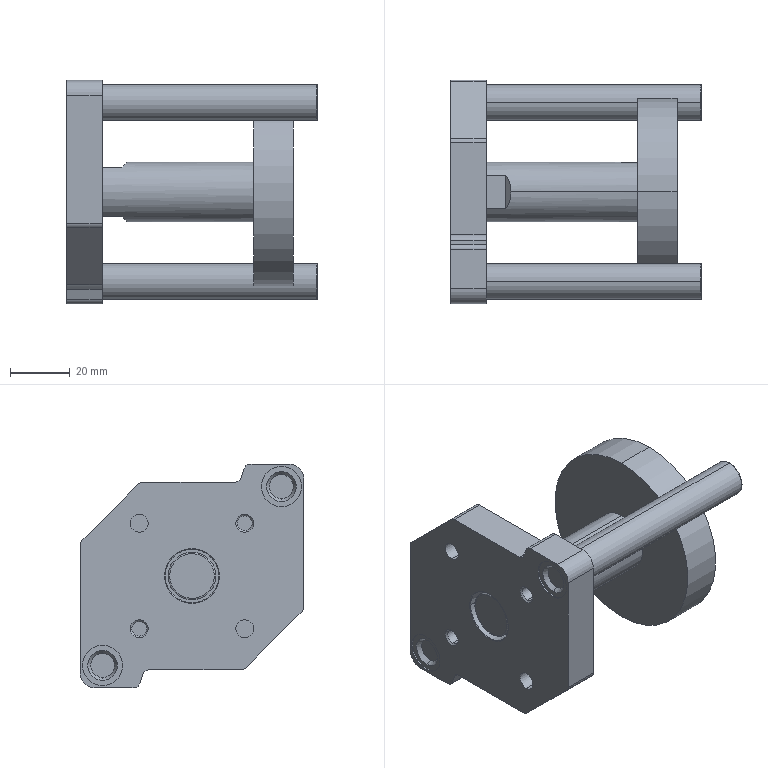Part | SolidWorks | features BaseBody 1 | 1 solid | 80 faces | box 84.2 x 75 x 75 mm | volume 125817 mm3 | cylinder 34 | plane 26 | cone 14 | spline 6 | commonest cylinder face diameters 4 x8 4.917 x4 6 x4 12 x4 13.5 x4 10 x2